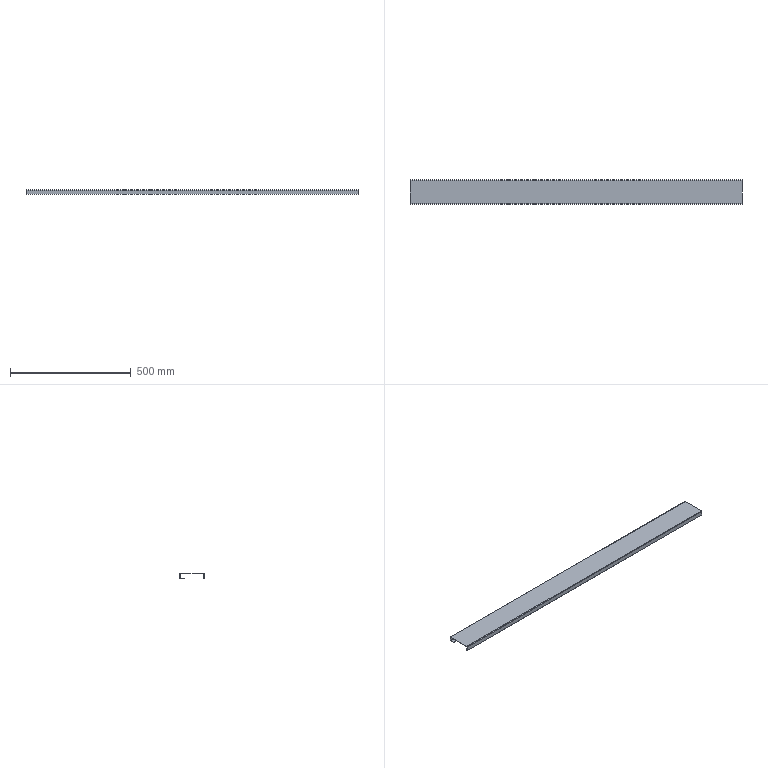Part | STEP file | E3-中转釜护栏6踢脚Plate | 1 solid | 18 faces | box 1375 x 100 x 20 mm | volume 316071 mm3 | plane 12 | cylinder 6 | commonest cylinder face diameters 2 x3 5 x3
STEP:
#1=CARTESIAN_POINT('',(0.,0.,0.));
#2=DIRECTION('',(0.,0.,1.));
#3=DIRECTION('',(1.,0.,0.));
#4=AXIS2_PLACEMENT_3D('',#1,#2,#3);
#5=CARTESIAN_POINT('',(-687.5,1.5,-2.5));
#6=VERTEX_POINT('',#5);
#7=CARTESIAN_POINT('',(-687.5,1.5,-20.));
#8=VERTEX_POINT('',#7);
#9=CARTESIAN_POINT('',(-687.5,1.5,-2.5));
#10=DIRECTION('',(0.,0.,-1.));
#11=VECTOR('',#10,1.);
#12=LINE('',#9,#11);
#13=CARTESIAN_POINT('',(687.5,1.5,-2.5));
#14=DIRECTION('',(0.,-1.,0.));
#15=DIRECTION('',(0.,0.,1.));
#16=AXIS2_PLACEMENT_3D('',#13,#14,#15);
#17=PLANE('',#16);
#18=CARTESIAN_POINT('',(0.,1375.));
#19=DIRECTION('',(-1.,0.));
#20=VECTOR('',#19,1.);
#21=LINE('',#18,#20);
#22=(GEOMETRIC_REPRESENTATION_CONTEXT(2)PARAMETRIC_REPRESENTATION_CONTEXT()REPRESENTATION_CONTEXT('',''));
#23=DEFINITIONAL_REPRESENTATION('',(#21),#22);
#24=PCURVE('',#17,#23);
#25=CARTESIAN_POINT('',(-687.5,2.5,-2.5));
#26=DIRECTION('',(-1.,0.,0.));
#27=DIRECTION('',(0.,0.,-1.));
#28=AXIS2_PLACEMENT_3D('',#25,#26,#27);
#29=PLANE('',#28);
#30=CARTESIAN_POINT('',(0.,1.));
#31=DIRECTION('',(1.,0.));
#32=VECTOR('',#31,1.);
#33=LINE('',#30,#32);
#34=(GEOMETRIC_REPRESENTATION_CONTEXT(2)PARAMETRIC_REPRESENTATION_CONTEXT()REPRESENTATION_CONTEXT('',''));
#35=DEFINITIONAL_REPRESENTATION('',(#33),#34);
#36=PCURVE('',#29,#35);
#37=SURFACE_CURVE('',#12,(#24,#36),.PCURVE_S1.);
#38=EDGE_CURVE('',#6,#8,#37,.T.);
#39=ORIENTED_EDGE('',*,*,#38,.F.);
#40=CARTESIAN_POINT('',(687.5,1.5,-2.5));
#41=VERTEX_POINT('',#40);
#42=CARTESIAN_POINT('',(687.5,1.5,-2.5));
#43=DIRECTION('',(-1.,0.,0.));
#44=VECTOR('',#43,1.);
#45=LINE('',#42,#44);
#46=CARTESIAN_POINT('',(0.,0.));
#47=DIRECTION('',(0.,1.));
#48=VECTOR('',#47,1.);
#49=LINE('',#46,#48);
#50=(GEOMETRIC_REPRESENTATION_CONTEXT(2)PARAMETRIC_REPRESENTATION_CONTEXT()REPRESENTATION_CONTEXT('',''));
#51=DEFINITIONAL_REPRESENTATION('',(#49),#50);
#52=PCURVE('',#17,#51);
#53=CARTESIAN_POINT('',(687.5,2.5,-2.5));
#54=DIRECTION('',(-1.,0.,0.));
#55=DIRECTION('',(0.,0.,-1.));
#56=AXIS2_PLACEMENT_3D('',#53,#54,#55);
#57=CYLINDRICAL_SURFACE('',#56,1.);
#58=CARTESIAN_POINT('',(1.571,0.));
#59=DIRECTION('',(0.,1.));
#60=VECTOR('',#59,1.);
#61=LINE('',#58,#60);
#62=(GEOMETRIC_REPRESENTATION_CONTEXT(2)PARAMETRIC_REPRESENTATION_CONTEXT()REPRESENTATION_CONTEXT('',''));
#63=DEFINITIONAL_REPRESENTATION('',(#61),#62);
#64=PCURVE('',#57,#63);
#65=SURFACE_CURVE('',#45,(#52,#64),.PCURVE_S1.);
#66=EDGE_CURVE('',#41,#6,#65,.T.);
#67=ORIENTED_EDGE('',*,*,#66,.F.);
#68=CARTESIAN_POINT('',(687.5,1.5,-20.));
#69=VERTEX_POINT('',#68);
#70=CARTESIAN_POINT('',(687.5,1.5,-2.5));
#71=DIRECTION('',(0.,0.,-1.));
#72=VECTOR('',#71,1.);
#73=LINE('',#70,#72);
#74=CARTESIAN_POINT('',(0.,0.));
#75=DIRECTION('',(-1.,0.));
#76=VECTOR('',#75,1.);
#77=LINE('',#74,#76);
#78=(GEOMETRIC_REPRESENTATION_CONTEXT(2)PARAMETRIC_REPRESENTATION_CONTEXT()REPRESENTATION_CONTEXT('',''));
#79=DEFINITIONAL_REPRESENTATION('',(#77),#78);
#80=PCURVE('',#17,#79);
#81=CARTESIAN_POINT('',(687.5,2.5,-2.5));
#82=DIRECTION('',(-1.,0.,0.));
#83=DIRECTION('',(0.,0.,-1.));
#84=AXIS2_PLACEMENT_3D('',#81,#82,#83);
#85=PLANE('',#84);
#86=CARTESIAN_POINT('',(0.,1.));
#87=DIRECTION('',(1.,0.));
#88=VECTOR('',#87,1.);
#89=LINE('',#86,#88);
#90=(GEOMETRIC_REPRESENTATION_CONTEXT(2)PARAMETRIC_REPRESENTATION_CONTEXT()REPRESENTATION_CONTEXT('',''));
#91=DEFINITIONAL_REPRESENTATION('',(#89),#90);
#92=PCURVE('',#85,#91);
#93=SURFACE_CURVE('',#73,(#80,#92),.PCURVE_S1.);
#94=EDGE_CURVE('',#41,#69,#93,.T.);
#95=ORIENTED_EDGE('',*,*,#94,.T.);
#96=CARTESIAN_POINT('',(687.5,1.5,-20.));
#97=DIRECTION('',(-1.,0.,0.));
#98=VECTOR('',#97,1.);
#99=LINE('',#96,#98);
#100=CARTESIAN_POINT('',(-17.5,0.));
#101=DIRECTION('',(0.,1.));
#102=VECTOR('',#101,1.);
#103=LINE('',#100,#102);
#104=(GEOMETRIC_REPRESENTATION_CONTEXT(2)PARAMETRIC_REPRESENTATION_CONTEXT()REPRESENTATION_CONTEXT('',''));
#105=DEFINITIONAL_REPRESENTATION('',(#103),#104);
#106=PCURVE('',#17,#105);
#107=CARTESIAN_POINT('',(687.5,0.,-20.));
#108=DIRECTION('',(0.,0.,-1.));
#109=DIRECTION('',(1.,0.,0.));
#110=AXIS2_PLACEMENT_3D('',#107,#108,#109);
#111=PLANE('',#110);
#112=CARTESIAN_POINT('',(0.,-1.5));
#113=DIRECTION('',(-1.,0.));
#114=VECTOR('',#113,1.);
#115=LINE('',#112,#114);
#116=(GEOMETRIC_REPRESENTATION_CONTEXT(2)PARAMETRIC_REPRESENTATION_CONTEXT()REPRESENTATION_CONTEXT('',''));
#117=DEFINITIONAL_REPRESENTATION('',(#115),#116);
#118=PCURVE('',#111,#117);
#119=SURFACE_CURVE('',#99,(#106,#118),.PCURVE_S1.);
#120=EDGE_CURVE('',#69,#8,#119,.T.);
#121=ORIENTED_EDGE('',*,*,#120,.T.);
#122=EDGE_LOOP('',(#39,#67,#95,#121));
#123=FACE_BOUND('',#122,.T.);
#124=ADVANCED_FACE('',(#123),#17,.F.);
#125=CARTESIAN_POINT('',(-687.5,0.,-20.));
#126=VERTEX_POINT('',#125);
#127=CARTESIAN_POINT('',(-687.5,0.,-20.));
#128=DIRECTION('',(0.,1.,0.));
#129=VECTOR('',#128,1.);
#130=LINE('',#127,#129);
#131=CARTESIAN_POINT('',(-1375.,0.));
#132=DIRECTION('',(0.,-1.));
#133=VECTOR('',#132,1.);
#134=LINE('',#131,#133);
#135=(GEOMETRIC_REPRESENTATION_CONTEXT(2)PARAMETRIC_REPRESENTATION_CONTEXT()REPRESENTATION_CONTEXT('',''));
#136=DEFINITIONAL_REPRESENTATION('',(#134),#135);
#137=PCURVE('',#111,#136);
#138=CARTESIAN_POINT('',(17.5,2.5));
#139=DIRECTION('',(0.,-1.));
#140=VECTOR('',#139,1.);
#141=LINE('',#138,#140);
#142=(GEOMETRIC_REPRESENTATION_CONTEXT(2)PARAMETRIC_REPRESENTATION_CONTEXT()REPRESENTATION_CONTEXT('',''));
#143=DEFINITIONAL_REPRESENTATION('',(#141),#142);
#144=PCURVE('',#29,#143);
#145=SURFACE_CURVE('',#130,(#137,#144),.PCURVE_S1.);
#146=EDGE_CURVE('',#126,#8,#145,.T.);
#147=ORIENTED_EDGE('',*,*,#146,.T.);
#148=ORIENTED_EDGE('',*,*,#120,.F.);
#149=CARTESIAN_POINT('',(687.5,0.,-20.));
#150=VERTEX_POINT('',#149);
#151=CARTESIAN_POINT('',(687.5,0.,-20.));
#152=DIRECTION('',(0.,1.,0.));
#153=VECTOR('',#152,1.);
#154=LINE('',#151,#153);
#155=CARTESIAN_POINT('',(0.,0.));
#156=DIRECTION('',(0.,-1.));
#157=VECTOR('',#156,1.);
#158=LINE('',#155,#157);
#159=(GEOMETRIC_REPRESENTATION_CONTEXT(2)PARAMETRIC_REPRESENTATION_CONTEXT()REPRESENTATION_CONTEXT('',''));
#160=DEFINITIONAL_REPRESENTATION('',(#158),#159);
#161=PCURVE('',#111,#160);
#162=CARTESIAN_POINT('',(17.5,2.5));
#163=DIRECTION('',(0.,-1.));
#164=VECTOR('',#163,1.);
#165=LINE('',#162,#164);
#166=(GEOMETRIC_REPRESENTATION_CONTEXT(2)PARAMETRIC_REPRESENTATION_CONTEXT()REPRESENTATION_CONTEXT('',''));
#167=DEFINITIONAL_REPRESENTATION('',(#165),#166);
#168=PCURVE('',#85,#167);
#169=SURFACE_CURVE('',#154,(#161,#168),.PCURVE_S1.);
#170=EDGE_CURVE('',#150,#69,#169,.T.);
#171=ORIENTED_EDGE('',*,*,#170,.F.);
#172=CARTESIAN_POINT('',(687.5,0.,-20.));
#173=DIRECTION('',(-1.,0.,0.));
#174=VECTOR('',#173,1.);
#175=LINE('',#172,#174);
#176=CARTESIAN_POINT('',(0.,0.));
#177=DIRECTION('',(-1.,0.));
#178=VECTOR('',#177,1.);
#179=LINE('',#176,#178);
#180=(GEOMETRIC_REPRESENTATION_CONTEXT(2)PARAMETRIC_REPRESENTATION_CONTEXT()REPRESENTATION_CONTEXT('',''));
#181=DEFINITIONAL_REPRESENTATION('',(#179),#180);
#182=PCURVE('',#111,#181);
#183=CARTESIAN_POINT('',(687.5,0.,-2.5));
#184=DIRECTION('',(0.,-1.,0.));
#185=DIRECTION('',(0.,0.,1.));
#186=AXIS2_PLACEMENT_3D('',#183,#184,#185);
#187=PLANE('',#186);
#188=CARTESIAN_POINT('',(-17.5,0.));
#189=DIRECTION('',(0.,1.));
#190=VECTOR('',#189,1.);
#191=LINE('',#188,#190);
#192=(GEOMETRIC_REPRESENTATION_CONTEXT(2)PARAMETRIC_REPRESENTATION_CONTEXT()REPRESENTATION_CONTEXT('',''));
#193=DEFINITIONAL_REPRESENTATION('',(#191),#192);
#194=PCURVE('',#187,#193);
#195=SURFACE_CURVE('',#175,(#182,#194),.PCURVE_S1.);
#196=EDGE_CURVE('',#150,#126,#195,.T.);
#197=ORIENTED_EDGE('',*,*,#196,.T.);
#198=EDGE_LOOP('',(#147,#148,#171,#197));
#199=FACE_BOUND('',#198,.T.);
#200=ADVANCED_FACE('',(#199),#111,.T.);
#201=CARTESIAN_POINT('',(-687.5,0.,-2.5));
#202=VERTEX_POINT('',#201);
#203=CARTESIAN_POINT('',(-687.5,0.,-2.5));
#204=DIRECTION('',(0.,0.,-1.));
#205=VECTOR('',#204,1.);
#206=LINE('',#203,#205);
#207=CARTESIAN_POINT('',(0.,1375.));
#208=DIRECTION('',(-1.,0.));
#209=VECTOR('',#208,1.);
#210=LINE('',#207,#209);
#211=(GEOMETRIC_REPRESENTATION_CONTEXT(2)PARAMETRIC_REPRESENTATION_CONTEXT()REPRESENTATION_CONTEXT('',''));
#212=DEFINITIONAL_REPRESENTATION('',(#210),#211);
#213=PCURVE('',#187,#212);
#214=CARTESIAN_POINT('',(0.,2.5));
#215=DIRECTION('',(1.,0.));
#216=VECTOR('',#215,1.);
#217=LINE('',#214,#216);
#218=(GEOMETRIC_REPRESENTATION_CONTEXT(2)PARAMETRIC_REPRESENTATION_CONTEXT()REPRESENTATION_CONTEXT('',''));
#219=DEFINITIONAL_REPRESENTATION('',(#217),#218);
#220=PCURVE('',#29,#219);
#221=SURFACE_CURVE('',#206,(#213,#220),.PCURVE_S1.);
#222=EDGE_CURVE('',#202,#126,#221,.T.);
#223=ORIENTED_EDGE('',*,*,#222,.T.);
#224=ORIENTED_EDGE('',*,*,#196,.F.);
#225=CARTESIAN_POINT('',(687.5,0.,-2.5));
#226=VERTEX_POINT('',#225);
#227=CARTESIAN_POINT('',(687.5,0.,-2.5));
#228=DIRECTION('',(0.,0.,-1.));
#229=VECTOR('',#228,1.);
#230=LINE('',#227,#229);
#231=CARTESIAN_POINT('',(0.,0.));
#232=DIRECTION('',(-1.,0.));
#233=VECTOR('',#232,1.);
#234=LINE('',#231,#233);
#235=(GEOMETRIC_REPRESENTATION_CONTEXT(2)PARAMETRIC_REPRESENTATION_CONTEXT()REPRESENTATION_CONTEXT('',''));
#236=DEFINITIONAL_REPRESENTATION('',(#234),#235);
#237=PCURVE('',#187,#236);
#238=CARTESIAN_POINT('',(0.,2.5));
#239=DIRECTION('',(1.,0.));
#240=VECTOR('',#239,1.);
#241=LINE('',#238,#240);
#242=(GEOMETRIC_REPRESENTATION_CONTEXT(2)PARAMETRIC_REPRESENTATION_CONTEXT()REPRESENTATION_CONTEXT('',''));
#243=DEFINITIONAL_REPRESENTATION('',(#241),#242);
#244=PCURVE('',#85,#243);
#245=SURFACE_CURVE('',#230,(#237,#244),.PCURVE_S1.);
#246=EDGE_CURVE('',#226,#150,#245,.T.);
#247=ORIENTED_EDGE('',*,*,#246,.F.);
#248=CARTESIAN_POINT('',(687.5,0.,-2.5));
#249=DIRECTION('',(-1.,0.,0.));
#250=VECTOR('',#249,1.);
#251=LINE('',#248,#250);
#252=CARTESIAN_POINT('',(0.,0.));
#253=DIRECTION('',(0.,1.));
#254=VECTOR('',#253,1.);
#255=LINE('',#252,#254);
#256=(GEOMETRIC_REPRESENTATION_CONTEXT(2)PARAMETRIC_REPRESENTATION_CONTEXT()REPRESENTATION_CONTEXT('',''));
#257=DEFINITIONAL_REPRESENTATION('',(#255),#256);
#258=PCURVE('',#187,#257);
#259=CARTESIAN_POINT('',(687.5,2.5,-2.5));
#260=DIRECTION('',(-1.,0.,0.));
#261=DIRECTION('',(0.,0.,-1.));
#262=AXIS2_PLACEMENT_3D('',#259,#260,#261);
#263=CYLINDRICAL_SURFACE('',#262,2.5);
#264=CARTESIAN_POINT('',(1.571,0.));
#265=DIRECTION('',(0.,1.));
#266=VECTOR('',#265,1.);
#267=LINE('',#264,#266);
#268=(GEOMETRIC_REPRESENTATION_CONTEXT(2)PARAMETRIC_REPRESENTATION_CONTEXT()REPRESENTATION_CONTEXT('',''));
#269=DEFINITIONAL_REPRESENTATION('',(#267),#268);
#270=PCURVE('',#263,#269);
#271=SURFACE_CURVE('',#251,(#258,#270),.PCURVE_S1.);
#272=EDGE_CURVE('',#226,#202,#271,.T.);
#273=ORIENTED_EDGE('',*,*,#272,.T.);
#274=EDGE_LOOP('',(#223,#224,#247,#273));
#275=FACE_BOUND('',#274,.T.);
#276=ADVANCED_FACE('',(#275),#187,.T.);
#277=CARTESIAN_POINT('',(-687.5,2.5,0.));
#278=VERTEX_POINT('',#277);
#279=CARTESIAN_POINT('',(-687.5,2.5,-2.5));
#280=DIRECTION('',(1.,0.,0.));
#281=DIRECTION('',(0.,0.,-1.));
#282=AXIS2_PLACEMENT_3D('',#279,#280,#281);
#283=CIRCLE('',#282,2.5);
#284=CARTESIAN_POINT('',(6.283,1375.));
#285=DIRECTION('',(-1.,0.));
#286=VECTOR('',#285,1.);
#287=LINE('',#284,#286);
#288=(GEOMETRIC_REPRESENTATION_CONTEXT(2)PARAMETRIC_REPRESENTATION_CONTEXT()REPRESENTATION_CONTEXT('',''));
#289=DEFINITIONAL_REPRESENTATION('',(#287),#288);
#290=PCURVE('',#263,#289);
#291=CARTESIAN_POINT('',(2.5,0.));
#292=CARTESIAN_POINT('',(2.5,-4.33));
#293=CARTESIAN_POINT('',(-1.25,-2.165));
#294=CARTESIAN_POINT('',(-5.,0.));
#295=CARTESIAN_POINT('',(-1.25,2.165));
#296=CARTESIAN_POINT('',(2.5,4.33));
#297=CARTESIAN_POINT('',(2.5,0.));
#298=(BOUNDED_CURVE()B_SPLINE_CURVE(2,(#291,#292,#293,#294,#295,#296,#297),.UNSPECIFIED.,.T.,.F.)B_SPLINE_CURVE_WITH_KNOTS((1,2,2,2,2,1),(-2.094,0.,2.094,4.189,6.283,8.378),.UNSPECIFIED.)CURVE()GEOMETRIC_REPRESENTATION_ITEM()RATIONAL_B_SPLINE_CURVE((1.,0.5,1.,0.5,1.,0.5,1.))REPRESENTATION_ITEM(''));
#299=(GEOMETRIC_REPRESENTATION_CONTEXT(2)PARAMETRIC_REPRESENTATION_CONTEXT()REPRESENTATION_CONTEXT('',''));
#300=DEFINITIONAL_REPRESENTATION('',(#298),#299);
#301=PCURVE('',#29,#300);
#302=SURFACE_CURVE('',#283,(#290,#301),.PCURVE_S1.);
#303=EDGE_CURVE('',#278,#202,#302,.T.);
#304=ORIENTED_EDGE('',*,*,#303,.T.);
#305=ORIENTED_EDGE('',*,*,#272,.F.);
#306=CARTESIAN_POINT('',(687.5,2.5,0.));
#307=VERTEX_POINT('',#306);
#308=CARTESIAN_POINT('',(687.5,2.5,-2.5));
#309=DIRECTION('',(1.,0.,0.));
#310=DIRECTION('',(0.,0.,-1.));
#311=AXIS2_PLACEMENT_3D('',#308,#309,#310);
#312=CIRCLE('',#311,2.5);
#313=CARTESIAN_POINT('',(6.283,0.));
#314=DIRECTION('',(-1.,0.));
#315=VECTOR('',#314,1.);
#316=LINE('',#313,#315);
#317=(GEOMETRIC_REPRESENTATION_CONTEXT(2)PARAMETRIC_REPRESENTATION_CONTEXT()REPRESENTATION_CONTEXT('',''));
#318=DEFINITIONAL_REPRESENTATION('',(#316),#317);
#319=PCURVE('',#263,#318);
#320=CARTESIAN_POINT('',(2.5,0.));
#321=CARTESIAN_POINT('',(2.5,-4.33));
#322=CARTESIAN_POINT('',(-1.25,-2.165));
#323=CARTESIAN_POINT('',(-5.,0.));
#324=CARTESIAN_POINT('',(-1.25,2.165));
#325=CARTESIAN_POINT('',(2.5,4.33));
#326=CARTESIAN_POINT('',(2.5,0.));
#327=(BOUNDED_CURVE()B_SPLINE_CURVE(2,(#320,#321,#322,#323,#324,#325,#326),.UNSPECIFIED.,.T.,.F.)B_SPLINE_CURVE_WITH_KNOTS((1,2,2,2,2,1),(-2.094,0.,2.094,4.189,6.283,8.378),.UNSPECIFIED.)CURVE()GEOMETRIC_REPRESENTATION_ITEM()RATIONAL_B_SPLINE_CURVE((1.,0.5,1.,0.5,1.,0.5,1.))REPRESENTATION_ITEM(''));
#328=(GEOMETRIC_REPRESENTATION_CONTEXT(2)PARAMETRIC_REPRESENTATION_CONTEXT()REPRESENTATION_CONTEXT('',''));
#329=DEFINITIONAL_REPRESENTATION('',(#327),#328);
#330=PCURVE('',#85,#329);
#331=SURFACE_CURVE('',#312,(#319,#330),.PCURVE_S1.);
#332=EDGE_CURVE('',#307,#226,#331,.T.);
#333=ORIENTED_EDGE('',*,*,#332,.F.);
#334=CARTESIAN_POINT('',(687.5,2.5,0.));
#335=DIRECTION('',(-1.,0.,0.));
#336=VECTOR('',#335,1.);
#337=LINE('',#334,#336);
#338=CARTESIAN_POINT('',(3.142,0.));
#339=DIRECTION('',(0.,1.));
#340=VECTOR('',#339,1.);
#341=LINE('',#338,#340);
#342=(GEOMETRIC_REPRESENTATION_CONTEXT(2)PARAMETRIC_REPRESENTATION_CONTEXT()REPRESENTATION_CONTEXT('',''));
#343=DEFINITIONAL_REPRESENTATION('',(#341),#342);
#344=PCURVE('',#263,#343);
#345=CARTESIAN_POINT('',(687.5,2.5,0.));
#346=DIRECTION('',(0.,0.,1.));
#347=DIRECTION('',(-1.,0.,0.));
#348=AXIS2_PLACEMENT_3D('',#345,#346,#347);
#349=PLANE('',#348);
#350=CARTESIAN_POINT('',(0.,0.));
#351=DIRECTION('',(1.,0.));
#352=VECTOR('',#351,1.);
#353=LINE('',#350,#352);
#354=(GEOMETRIC_REPRESENTATION_CONTEXT(2)PARAMETRIC_REPRESENTATION_CONTEXT()REPRESENTATION_CONTEXT('',''));
#355=DEFINITIONAL_REPRESENTATION('',(#353),#354);
#356=PCURVE('',#349,#355);
#357=SURFACE_CURVE('',#337,(#344,#356),.PCURVE_S1.);
#358=EDGE_CURVE('',#307,#278,#357,.T.);
#359=ORIENTED_EDGE('',*,*,#358,.T.);
#360=EDGE_LOOP('',(#304,#305,#333,#359));
#361=FACE_BOUND('',#360,.T.);
#362=ADVANCED_FACE('',(#361),#263,.T.);
#363=CARTESIAN_POINT('',(-687.5,97.5,0.));
#364=VERTEX_POINT('',#363);
#365=CARTESIAN_POINT('',(-687.5,2.5,0.));
#366=DIRECTION('',(0.,-1.,0.));
#367=VECTOR('',#366,1.);
#368=LINE('',#365,#367);
#369=CARTESIAN_POINT('',(1375.,0.));
#370=DIRECTION('',(0.,1.));
#371=VECTOR('',#370,1.);
#372=LINE('',#369,#371);
#373=(GEOMETRIC_REPRESENTATION_CONTEXT(2)PARAMETRIC_REPRESENTATION_CONTEXT()REPRESENTATION_CONTEXT('',''));
#374=DEFINITIONAL_REPRESENTATION('',(#372),#373);
#375=PCURVE('',#349,#374);
#376=CARTESIAN_POINT('',(-2.5,0.));
#377=DIRECTION('',(0.,1.));
#378=VECTOR('',#377,1.);
#379=LINE('',#376,#378);
#380=(GEOMETRIC_REPRESENTATION_CONTEXT(2)PARAMETRIC_REPRESENTATION_CONTEXT()REPRESENTATION_CONTEXT('',''));
#381=DEFINITIONAL_REPRESENTATION('',(#379),#380);
#382=PCURVE('',#29,#381);
#383=SURFACE_CURVE('',#368,(#375,#382),.PCURVE_S1.);
#384=EDGE_CURVE('',#364,#278,#383,.T.);
#385=ORIENTED_EDGE('',*,*,#384,.T.);
#386=ORIENTED_EDGE('',*,*,#358,.F.);
#387=CARTESIAN_POINT('',(687.5,97.5,0.));
#388=VERTEX_POINT('',#387);
#389=CARTESIAN_POINT('',(687.5,2.5,0.));
#390=DIRECTION('',(0.,-1.,0.));
#391=VECTOR('',#390,1.);
#392=LINE('',#389,#391);
#393=CARTESIAN_POINT('',(0.,0.));
#394=DIRECTION('',(0.,1.));
#395=VECTOR('',#394,1.);
#396=LINE('',#393,#395);
#397=(GEOMETRIC_REPRESENTATION_CONTEXT(2)PARAMETRIC_REPRESENTATION_CONTEXT()REPRESENTATION_CONTEXT('',''));
#398=DEFINITIONAL_REPRESENTATION('',(#396),#397);
#399=PCURVE('',#349,#398);
#400=CARTESIAN_POINT('',(-2.5,0.));
#401=DIRECTION('',(0.,1.));
#402=VECTOR('',#401,1.);
#403=LINE('',#400,#402);
#404=(GEOMETRIC_REPRESENTATION_CONTEXT(2)PARAMETRIC_REPRESENTATION_CONTEXT()REPRESENTATION_CONTEXT('',''));
#405=DEFINITIONAL_REPRESENTATION('',(#403),#404);
#406=PCURVE('',#85,#405);
#407=SURFACE_CURVE('',#392,(#399,#406),.PCURVE_S1.);
#408=EDGE_CURVE('',#388,#307,#407,.T.);
#409=ORIENTED_EDGE('',*,*,#408,.F.);
#410=CARTESIAN_POINT('',(687.5,97.5,0.));
#411=DIRECTION('',(-1.,0.,0.));
#412=VECTOR('',#411,1.);
#413=LINE('',#410,#412);
#414=CARTESIAN_POINT('',(0.,-95.));
#415=DIRECTION('',(1.,0.));
#416=VECTOR('',#415,1.);
#417=LINE('',#414,#416);
#418=(GEOMETRIC_REPRESENTATION_CONTEXT(2)PARAMETRIC_REPRESENTATION_CONTEXT()REPRESENTATION_CONTEXT('',''));
#419=DEFINITIONAL_REPRESENTATION('',(#417),#418);
#420=PCURVE('',#349,#419);
#421=CARTESIAN_POINT('',(687.5,97.5,-2.5));
#422=DIRECTION('',(-1.,0.,0.));
#423=DIRECTION('',(0.,0.,-1.));
#424=AXIS2_PLACEMENT_3D('',#421,#422,#423);
#425=CYLINDRICAL_SURFACE('',#424,2.5);
#426=CARTESIAN_POINT('',(3.142,0.));
#427=DIRECTION('',(0.,1.));
#428=VECTOR('',#427,1.);
#429=LINE('',#426,#428);
#430=(GEOMETRIC_REPRESENTATION_CONTEXT(2)PARAMETRIC_REPRESENTATION_CONTEXT()REPRESENTATION_CONTEXT('',''));
#431=DEFINITIONAL_REPRESENTATION('',(#429),#430);
#432=PCURVE('',#425,#431);
#433=SURFACE_CURVE('',#413,(#420,#432),.PCURVE_S1.);
#434=EDGE_CURVE('',#388,#364,#433,.T.);
#435=ORIENTED_EDGE('',*,*,#434,.T.);
#436=EDGE_LOOP('',(#385,#386,#409,#435));
#437=FACE_BOUND('',#436,.T.);
#438=ADVANCED_FACE('',(#437),#349,.T.);
#439=CARTESIAN_POINT('',(-687.5,100.,-2.5));
#440=VERTEX_POINT('',#439);
#441=CARTESIAN_POINT('',(-687.5,97.5,-2.5));
#442=DIRECTION('',(1.,0.,0.));
#443=DIRECTION('',(0.,0.,1.));
#444=AXIS2_PLACEMENT_3D('',#441,#442,#443);
#445=CIRCLE('',#444,2.5);
#446=CARTESIAN_POINT('',(9.425,1375.));
#447=DIRECTION('',(-1.,0.));
#448=VECTOR('',#447,1.);
#449=LINE('',#446,#448);
#450=(GEOMETRIC_REPRESENTATION_CONTEXT(2)PARAMETRIC_REPRESENTATION_CONTEXT()REPRESENTATION_CONTEXT('',''));
#451=DEFINITIONAL_REPRESENTATION('',(#449),#450);
#452=PCURVE('',#425,#451);
#453=CARTESIAN_POINT('',(-2.5,-95.));
#454=CARTESIAN_POINT('',(-2.5,-90.67));
#455=CARTESIAN_POINT('',(1.25,-92.835));
#456=CARTESIAN_POINT('',(5.,-95.));
#457=CARTESIAN_POINT('',(1.25,-97.165));
#458=CARTESIAN_POINT('',(-2.5,-99.33));
#459=CARTESIAN_POINT('',(-2.5,-95.));
#460=(BOUNDED_CURVE()B_SPLINE_CURVE(2,(#453,#454,#455,#456,#457,#458,#459),.UNSPECIFIED.,.T.,.F.)B_SPLINE_CURVE_WITH_KNOTS((1,2,2,2,2,1),(-2.094,0.,2.094,4.189,6.283,8.378),.UNSPECIFIED.)CURVE()GEOMETRIC_REPRESENTATION_ITEM()RATIONAL_B_SPLINE_CURVE((1.,0.5,1.,0.5,1.,0.5,1.))REPRESENTATION_ITEM(''));
#461=(GEOMETRIC_REPRESENTATION_CONTEXT(2)PARAMETRIC_REPRESENTATION_CONTEXT()REPRESENTATION_CONTEXT('',''));
#462=DEFINITIONAL_REPRESENTATION('',(#460),#461);
#463=PCURVE('',#29,#462);
#464=SURFACE_CURVE('',#445,(#452,#463),.PCURVE_S1.);
#465=EDGE_CURVE('',#440,#364,#464,.T.);
#466=ORIENTED_EDGE('',*,*,#465,.T.);
#467=ORIENTED_EDGE('',*,*,#434,.F.);
#468=CARTESIAN_POINT('',(687.5,100.,-2.5));
#469=VERTEX_POINT('',#468);
#470=CARTESIAN_POINT('',(687.5,97.5,-2.5));
#471=DIRECTION('',(1.,0.,0.));
#472=DIRECTION('',(0.,0.,1.));
#473=AXIS2_PLACEMENT_3D('',#470,#471,#472);
#474=CIRCLE('',#473,2.5);
#475=CARTESIAN_POINT('',(9.425,0.));
#476=DIRECTION('',(-1.,0.));
#477=VECTOR('',#476,1.);
#478=LINE('',#475,#477);
#479=(GEOMETRIC_REPRESENTATION_CONTEXT(2)PARAMETRIC_REPRESENTATION_CONTEXT()REPRESENTATION_CONTEXT('',''));
#480=DEFINITIONAL_REPRESENTATION('',(#478),#479);
#481=PCURVE('',#425,#480);
#482=CARTESIAN_POINT('',(-2.5,-95.));
#483=CARTESIAN_POINT('',(-2.5,-90.67));
#484=CARTESIAN_POINT('',(1.25,-92.835));
#485=CARTESIAN_POINT('',(5.,-95.));
#486=CARTESIAN_POINT('',(1.25,-97.165));
#487=CARTESIAN_POINT('',(-2.5,-99.33));
#488=CARTESIAN_POINT('',(-2.5,-95.));
#489=(BOUNDED_CURVE()B_SPLINE_CURVE(2,(#482,#483,#484,#485,#486,#487,#488),.UNSPECIFIED.,.T.,.F.)B_SPLINE_CURVE_WITH_KNOTS((1,2,2,2,2,1),(-2.094,0.,2.094,4.189,6.283,8.378),.UNSPECIFIED.)CURVE()GEOMETRIC_REPRESENTATION_ITEM()RATIONAL_B_SPLINE_CURVE((1.,0.5,1.,0.5,1.,0.5,1.))REPRESENTATION_ITEM(''));
#490=(GEOMETRIC_REPRESENTATION_CONTEXT(2)PARAMETRIC_REPRESENTATION_CONTEXT()REPRESENTATION_CONTEXT('',''));
#491=DEFINITIONAL_REPRESENTATION('',(#489),#490);
#492=PCURVE('',#85,#491);
#493=SURFACE_CURVE('',#474,(#481,#492),.PCURVE_S1.);
#494=EDGE_CURVE('',#469,#388,#493,.T.);
#495=ORIENTED_EDGE('',*,*,#494,.F.);
#496=CARTESIAN_POINT('',(687.5,100.,-2.5));
#497=DIRECTION('',(-1.,0.,0.));
#498=VECTOR('',#497,1.);
#499=LINE('',#496,#498);
#500=CARTESIAN_POINT('',(4.712,0.));
#501=DIRECTION('',(0.,1.));
#502=VECTOR('',#501,1.);
#503=LINE('',#500,#502);
#504=(GEOMETRIC_REPRESENTATION_CONTEXT(2)PARAMETRIC_REPRESENTATION_CONTEXT()REPRESENTATION_CONTEXT('',''));
#505=DEFINITIONAL_REPRESENTATION('',(#503),#504);
#506=PCURVE('',#425,#505);
#507=CARTESIAN_POINT('',(687.5,100.,-2.5));
#508=DIRECTION('',(0.,1.,0.));
#509=DIRECTION('',(0.,0.,-1.));
#510=AXIS2_PLACEMENT_3D('',#507,#508,#509);
#511=PLANE('',#510);
#512=CARTESIAN_POINT('',(0.,0.));
#513=DIRECTION('',(0.,1.));
#514=VECTOR('',#513,1.);
#515=LINE('',#512,#514);
#516=(GEOMETRIC_REPRESENTATION_CONTEXT(2)PARAMETRIC_REPRESENTATION_CONTEXT()REPRESENTATION_CONTEXT('',''));
#517=DEFINITIONAL_REPRESENTATION('',(#515),#516);
#518=PCURVE('',#511,#517);
#519=SURFACE_CURVE('',#499,(#506,#518),.PCURVE_S1.);
#520=EDGE_CURVE('',#469,#440,#519,.T.);
#521=ORIENTED_EDGE('',*,*,#520,.T.);
#522=EDGE_LOOP('',(#466,#467,#495,#521));
#523=FACE_BOUND('',#522,.T.);
#524=ADVANCED_FACE('',(#523),#425,.T.);
#525=CARTESIAN_POINT('',(-687.5,100.,-17.5));
#526=VERTEX_POINT('',#525);
#527=CARTESIAN_POINT('',(-687.5,100.,-2.5));
#528=DIRECTION('',(0.,0.,1.));
#529=VECTOR('',#528,1.);
#530=LINE('',#527,#529);
#531=CARTESIAN_POINT('',(0.,1375.));
#532=DIRECTION('',(-1.,0.));
#533=VECTOR('',#532,1.);
#534=LINE('',#531,#533);
#535=(GEOMETRIC_REPRESENTATION_CONTEXT(2)PARAMETRIC_REPRESENTATION_CONTEXT()REPRESENTATION_CONTEXT('',''));
#536=DEFINITIONAL_REPRESENTATION('',(#534),#535);
#537=PCURVE('',#511,#536);
#538=CARTESIAN_POINT('',(0.,-97.5));
#539=DIRECTION('',(-1.,0.));
#540=VECTOR('',#539,1.);
#541=LINE('',#538,#540);
#542=(GEOMETRIC_REPRESENTATION_CONTEXT(2)PARAMETRIC_REPRESENTATION_CONTEXT()REPRESENTATION_CONTEXT('',''));
#543=DEFINITIONAL_REPRESENTATION('',(#541),#542);
#544=PCURVE('',#29,#543);
#545=SURFACE_CURVE('',#530,(#537,#544),.PCURVE_S1.);
#546=EDGE_CURVE('',#526,#440,#545,.T.);
#547=ORIENTED_EDGE('',*,*,#546,.T.);
#548=ORIENTED_EDGE('',*,*,#520,.F.);
#549=CARTESIAN_POINT('',(687.5,100.,-17.5));
#550=VERTEX_POINT('',#549);
#551=CARTESIAN_POINT('',(687.5,100.,-2.5));
#552=DIRECTION('',(0.,0.,1.));
#553=VECTOR('',#552,1.);
#554=LINE('',#551,#553);
#555=CARTESIAN_POINT('',(0.,0.));
#556=DIRECTION('',(-1.,0.));
#557=VECTOR('',#556,1.);
#558=LINE('',#555,#557);
#559=(GEOMETRIC_REPRESENTATION_CONTEXT(2)PARAMETRIC_REPRESENTATION_CONTEXT()REPRESENTATION_CONTEXT('',''));
#560=DEFINITIONAL_REPRESENTATION('',(#558),#559);
#561=PCURVE('',#511,#560);
#562=CARTESIAN_POINT('',(0.,-97.5));
#563=DIRECTION('',(-1.,0.));
#564=VECTOR('',#563,1.);
#565=LINE('',#562,#564);
#566=(GEOMETRIC_REPRESENTATION_CONTEXT(2)PARAMETRIC_REPRESENTATION_CONTEXT()REPRESENTATION_CONTEXT('',''));
#567=DEFINITIONAL_REPRESENTATION('',(#565),#566);
#568=PCURVE('',#85,#567);
#569=SURFACE_CURVE('',#554,(#561,#568),.PCURVE_S1.);
#570=EDGE_CURVE('',#550,#469,#569,.T.);
#571=ORIENTED_EDGE('',*,*,#570,.F.);
#572=CARTESIAN_POINT('',(687.5,100.,-17.5));
#573=DIRECTION('',(-1.,0.,0.));
#574=VECTOR('',#573,1.);
#575=LINE('',#572,#574);
#576=CARTESIAN_POINT('',(15.,0.));
#577=DIRECTION('',(0.,1.));
#578=VECTOR('',#577,1.);
#579=LINE('',#576,#578);
#580=(GEOMETRIC_REPRESENTATION_CONTEXT(2)PARAMETRIC_REPRESENTATION_CONTEXT()REPRESENTATION_CONTEXT('',''));
#581=DEFINITIONAL_REPRESENTATION('',(#579),#580);
#582=PCURVE('',#511,#581);
#583=CARTESIAN_POINT('',(687.5,97.5,-17.5));
#584=DIRECTION('',(-1.,0.,0.));
#585=DIRECTION('',(0.,0.,-1.));
#586=AXIS2_PLACEMENT_3D('',#583,#584,#585);
#587=CYLINDRICAL_SURFACE('',#586,2.5);
#588=CARTESIAN_POINT('',(4.712,0.));
#589=DIRECTION('',(0.,1.));
#590=VECTOR('',#589,1.);
#591=LINE('',#588,#590);
#592=(GEOMETRIC_REPRESENTATION_CONTEXT(2)PARAMETRIC_REPRESENTATION_CONTEXT()REPRESENTATION_CONTEXT('',''));
#593=DEFINITIONAL_REPRESENTATION('',(#591),#592);
#594=PCURVE('',#587,#593);
#595=SURFACE_CURVE('',#575,(#582,#594),.PCURVE_S1.);
#596=EDGE_CURVE('',#550,#526,#595,.T.);
#597=ORIENTED_EDGE('',*,*,#596,.T.);
#598=EDGE_LOOP('',(#547,#548,#571,#597));
#599=FACE_BOUND('',#598,.T.);
#600=ADVANCED_FACE('',(#599),#511,.T.);
#601=CARTESIAN_POINT('',(-687.5,97.5,-20.));
#602=VERTEX_POINT('',#601);
#603=CARTESIAN_POINT('',(-687.5,97.5,-17.5));
#604=DIRECTION('',(1.,0.,0.));
#605=DIRECTION('',(0.,0.,1.));
#606=AXIS2_PLACEMENT_3D('',#603,#604,#605);
#607=CIRCLE('',#606,2.5);
#608=CARTESIAN_POINT('',(9.425,1375.));
#609=DIRECTION('',(-1.,0.));
#610=VECTOR('',#609,1.);
#611=LINE('',#608,#610);
#612=(GEOMETRIC_REPRESENTATION_CONTEXT(2)PARAMETRIC_REPRESENTATION_CONTEXT()REPRESENTATION_CONTEXT('',''));
#613=DEFINITIONAL_REPRESENTATION('',(#611),#612);
#614=PCURVE('',#587,#613);
#615=CARTESIAN_POINT('',(12.5,-95.));
#616=CARTESIAN_POINT('',(12.5,-90.67));
#617=CARTESIAN_POINT('',(16.25,-92.835));
#618=CARTESIAN_POINT('',(20.,-95.));
#619=CARTESIAN_POINT('',(16.25,-97.165));
#620=CARTESIAN_POINT('',(12.5,-99.33));
#621=CARTESIAN_POINT('',(12.5,-95.));
#622=(BOUNDED_CURVE()B_SPLINE_CURVE(2,(#615,#616,#617,#618,#619,#620,#621),.UNSPECIFIED.,.T.,.F.)B_SPLINE_CURVE_WITH_KNOTS((1,2,2,2,2,1),(-2.094,0.,2.094,4.189,6.283,8.378),.UNSPECIFIED.)CURVE()GEOMETRIC_REPRESENTATION_ITEM()RATIONAL_B_SPLINE_CURVE((1.,0.5,1.,0.5,1.,0.5,1.))REPRESENTATION_ITEM(''));
#623=(GEOMETRIC_REPRESENTATION_CONTEXT(2)PARAMETRIC_REPRESENTATION_CONTEXT()REPRESENTATION_CONTEXT('',''));
#624=DEFINITIONAL_REPRESENTATION('',(#622),#623);
#625=PCURVE('',#29,#624);
#626=SURFACE_CURVE('',#607,(#614,#625),.PCURVE_S1.);
#627=EDGE_CURVE('',#602,#526,#626,.T.);
#628=ORIENTED_EDGE('',*,*,#627,.T.);
#629=ORIENTED_EDGE('',*,*,#596,.F.);
#630=CARTESIAN_POINT('',(687.5,97.5,-20.));
#631=VERTEX_POINT('',#630);
#632=CARTESIAN_POINT('',(687.5,97.5,-17.5));
#633=DIRECTION('',(1.,0.,0.));
#634=DIRECTION('',(0.,0.,1.));
#635=AXIS2_PLACEMENT_3D('',#632,#633,#634);
#636=CIRCLE('',#635,2.5);
#637=CARTESIAN_POINT('',(9.425,0.));
#638=DIRECTION('',(-1.,0.));
#639=VECTOR('',#638,1.);
#640=LINE('',#637,#639);
#641=(GEOMETRIC_REPRESENTATION_CONTEXT(2)PARAMETRIC_REPRESENTATION_CONTEXT()REPRESENTATION_CONTEXT('',''));
#642=DEFINITIONAL_REPRESENTATION('',(#640),#641);
#643=PCURVE('',#587,#642);
#644=CARTESIAN_POINT('',(12.5,-95.));
#645=CARTESIAN_POINT('',(12.5,-90.67));
#646=CARTESIAN_POINT('',(16.25,-92.835));
#647=CARTESIAN_POINT('',(20.,-95.));
#648=CARTESIAN_POINT('',(16.25,-97.165));
#649=CARTESIAN_POINT('',(12.5,-99.33));
#650=CARTESIAN_POINT('',(12.5,-95.));
#651=(BOUNDED_CURVE()B_SPLINE_CURVE(2,(#644,#645,#646,#647,#648,#649,#650),.UNSPECIFIED.,.T.,.F.)B_SPLINE_CURVE_WITH_KNOTS((1,2,2,2,2,1),(-2.094,0.,2.094,4.189,6.283,8.378),.UNSPECIFIED.)CURVE()GEOMETRIC_REPRESENTATION_ITEM()RATIONAL_B_SPLINE_CURVE((1.,0.5,1.,0.5,1.,0.5,1.))REPRESENTATION_ITEM(''));
#652=(GEOMETRIC_REPRESENTATION_CONTEXT(2)PARAMETRIC_REPRESENTATION_CONTEXT()REPRESENTATION_CONTEXT('',''));
#653=DEFINITIONAL_REPRESENTATION('',(#651),#652);
#654=PCURVE('',#85,#653);
#655=SURFACE_CURVE('',#636,(#643,#654),.PCURVE_S1.);
#656=EDGE_CURVE('',#631,#550,#655,.T.);
#657=ORIENTED_EDGE('',*,*,#656,.F.);
#658=CARTESIAN_POINT('',(687.5,97.5,-20.));
#659=DIRECTION('',(-1.,0.,0.));
#660=VECTOR('',#659,1.);
#661=LINE('',#658,#660);
#662=CARTESIAN_POINT('',(6.283,0.));
#663=DIRECTION('',(0.,1.));
#664=VECTOR('',#663,1.);
#665=LINE('',#662,#664);
#666=(GEOMETRIC_REPRESENTATION_CONTEXT(2)PARAMETRIC_REPRESENTATION_CONTEXT()REPRESENTATION_CONTEXT('',''));
#667=DEFINITIONAL_REPRESENTATION('',(#665),#666);
#668=PCURVE('',#587,#667);
#669=CARTESIAN_POINT('',(687.5,97.5,-20.));
#670=DIRECTION('',(0.,0.,-1.));
#671=DIRECTION('',(1.,0.,0.));
#672=AXIS2_PLACEMENT_3D('',#669,#670,#671);
#673=PLANE('',#672);
#674=CARTESIAN_POINT('',(0.,0.));
#675=DIRECTION('',(-1.,0.));
#676=VECTOR('',#675,1.);
#677=LINE('',#674,#676);
#678=(GEOMETRIC_REPRESENTATION_CONTEXT(2)PARAMETRIC_REPRESENTATION_CONTEXT()REPRESENTATION_CONTEXT('',''));
#679=DEFINITIONAL_REPRESENTATION('',(#677),#678);
#680=PCURVE('',#673,#679);
#681=SURFACE_CURVE('',#661,(#668,#680),.PCURVE_S1.);
#682=EDGE_CURVE('',#631,#602,#681,.T.);
#683=ORIENTED_EDGE('',*,*,#682,.T.);
#684=EDGE_LOOP('',(#628,#629,#657,#683));
#685=FACE_BOUND('',#684,.T.);
#686=ADVANCED_FACE('',(#685),#587,.T.);
#687=CARTESIAN_POINT('',(-687.5,80.,-20.));
#688=VERTEX_POINT('',#687);
#689=CARTESIAN_POINT('',(-687.5,97.5,-20.));
#690=DIRECTION('',(0.,1.,0.));
#691=VECTOR('',#690,1.);
#692=LINE('',#689,#691);
#693=CARTESIAN_POINT('',(-1375.,0.));
#694=DIRECTION('',(0.,-1.));
#695=VECTOR('',#694,1.);
#696=LINE('',#693,#695);
#697=(GEOMETRIC_REPRESENTATION_CONTEXT(2)PARAMETRIC_REPRESENTATION_CONTEXT()REPRESENTATION_CONTEXT('',''));
#698=DEFINITIONAL_REPRESENTATION('',(#696),#697);
#699=PCURVE('',#673,#698);
#700=CARTESIAN_POINT('',(17.5,-95.));
#701=DIRECTION('',(0.,-1.));
#702=VECTOR('',#701,1.);
#703=LINE('',#700,#702);
#704=(GEOMETRIC_REPRESENTATION_CONTEXT(2)PARAMETRIC_REPRESENTATION_CONTEXT()REPRESENTATION_CONTEXT('',''));
#705=DEFINITIONAL_REPRESENTATION('',(#703),#704);
#706=PCURVE('',#29,#705);
#707=SURFACE_CURVE('',#692,(#699,#706),.PCURVE_S1.);
#708=EDGE_CURVE('',#688,#602,#707,.T.);
#709=ORIENTED_EDGE('',*,*,#708,.T.);
#710=ORIENTED_EDGE('',*,*,#682,.F.);
#711=CARTESIAN_POINT('',(687.5,80.,-20.));
#712=VERTEX_POINT('',#711);
#713=CARTESIAN_POINT('',(687.5,97.5,-20.));
#714=DIRECTION('',(0.,1.,0.));
#715=VECTOR('',#714,1.);
#716=LINE('',#713,#715);
#717=CARTESIAN_POINT('',(0.,0.));
#718=DIRECTION('',(0.,-1.));
#719=VECTOR('',#718,1.);
#720=LINE('',#717,#719);
#721=(GEOMETRIC_REPRESENTATION_CONTEXT(2)PARAMETRIC_REPRESENTATION_CONTEXT()REPRESENTATION_CONTEXT('',''));
#722=DEFINITIONAL_REPRESENTATION('',(#720),#721);
#723=PCURVE('',#673,#722);
#724=CARTESIAN_POINT('',(17.5,-95.));
#725=DIRECTION('',(0.,-1.));
#726=VECTOR('',#725,1.);
#727=LINE('',#724,#726);
#728=(GEOMETRIC_REPRESENTATION_CONTEXT(2)PARAMETRIC_REPRESENTATION_CONTEXT()REPRESENTATION_CONTEXT('',''));
#729=DEFINITIONAL_REPRESENTATION('',(#727),#728);
#730=PCURVE('',#85,#729);
#731=SURFACE_CURVE('',#716,(#723,#730),.PCURVE_S1.);
#732=EDGE_CURVE('',#712,#631,#731,.T.);
#733=ORIENTED_EDGE('',*,*,#732,.F.);
#734=CARTESIAN_POINT('',(687.5,80.,-20.));
#735=DIRECTION('',(-1.,0.,0.));
#736=VECTOR('',#735,1.);
#737=LINE('',#734,#736);
#738=CARTESIAN_POINT('',(0.,17.5));
#739=DIRECTION('',(-1.,0.));
#740=VECTOR('',#739,1.);
#741=LINE('',#738,#740);
#742=(GEOMETRIC_REPRESENTATION_CONTEXT(2)PARAMETRIC_REPRESENTATION_CONTEXT()REPRESENTATION_CONTEXT('',''));
#743=DEFINITIONAL_REPRESENTATION('',(#741),#742);
#744=PCURVE('',#673,#743);
#745=CARTESIAN_POINT('',(687.5,80.,-18.5));
#746=DIRECTION('',(0.,-1.,0.));
#747=DIRECTION('',(0.,0.,1.));
#748=AXIS2_PLACEMENT_3D('',#745,#746,#747);
#749=PLANE('',#748);
#750=CARTESIAN_POINT('',(-1.5,0.));
#751=DIRECTION('',(0.,1.));
#752=VECTOR('',#751,1.);
#753=LINE('',#750,#752);
#754=(GEOMETRIC_REPRESENTATION_CONTEXT(2)PARAMETRIC_REPRESENTATION_CONTEXT()REPRESENTATION_CONTEXT('',''));
#755=DEFINITIONAL_REPRESENTATION('',(#753),#754);
#756=PCURVE('',#749,#755);
#757=SURFACE_CURVE('',#737,(#744,#756),.PCURVE_S1.);
#758=EDGE_CURVE('',#712,#688,#757,.T.);
#759=ORIENTED_EDGE('',*,*,#758,.T.);
#760=EDGE_LOOP('',(#709,#710,#733,#759));
#761=FACE_BOUND('',#760,.T.);
#762=ADVANCED_FACE('',(#761),#673,.T.);
#763=CARTESIAN_POINT('',(-687.5,80.,-18.5));
#764=VERTEX_POINT('',#763);
#765=CARTESIAN_POINT('',(-687.5,80.,-18.5));
#766=DIRECTION('',(0.,0.,-1.));
#767=VECTOR('',#766,1.);
#768=LINE('',#765,#767);
#769=CARTESIAN_POINT('',(0.,1375.));
#770=DIRECTION('',(-1.,0.));
#771=VECTOR('',#770,1.);
#772=LINE('',#769,#771);
#773=(GEOMETRIC_REPRESENTATION_CONTEXT(2)PARAMETRIC_REPRESENTATION_CONTEXT()REPRESENTATION_CONTEXT('',''));
#774=DEFINITIONAL_REPRESENTATION('',(#772),#773);
#775=PCURVE('',#749,#774);
#776=CARTESIAN_POINT('',(16.,-77.5));
#777=DIRECTION('',(1.,0.));
#778=VECTOR('',#777,1.);
#779=LINE('',#776,#778);
#780=(GEOMETRIC_REPRESENTATION_CONTEXT(2)PARAMETRIC_REPRESENTATION_CONTEXT()REPRESENTATION_CONTEXT('',''));
#781=DEFINITIONAL_REPRESENTATION('',(#779),#780);
#782=PCURVE('',#29,#781);
#783=SURFACE_CURVE('',#768,(#775,#782),.PCURVE_S1.);
#784=EDGE_CURVE('',#764,#688,#783,.T.);
#785=ORIENTED_EDGE('',*,*,#784,.T.);
#786=ORIENTED_EDGE('',*,*,#758,.F.);
#787=CARTESIAN_POINT('',(687.5,80.,-18.5));
#788=VERTEX_POINT('',#787);
#789=CARTESIAN_POINT('',(687.5,80.,-18.5));
#790=DIRECTION('',(0.,0.,-1.));
#791=VECTOR('',#790,1.);
#792=LINE('',#789,#791);
#793=CARTESIAN_POINT('',(0.,0.));
#794=DIRECTION('',(-1.,0.));
#795=VECTOR('',#794,1.);
#796=LINE('',#793,#795);
#797=(GEOMETRIC_REPRESENTATION_CONTEXT(2)PARAMETRIC_REPRESENTATION_CONTEXT()REPRESENTATION_CONTEXT('',''));
#798=DEFINITIONAL_REPRESENTATION('',(#796),#797);
#799=PCURVE('',#749,#798);
#800=CARTESIAN_POINT('',(16.,-77.5));
#801=DIRECTION('',(1.,0.));
#802=VECTOR('',#801,1.);
#803=LINE('',#800,#802);
#804=(GEOMETRIC_REPRESENTATION_CONTEXT(2)PARAMETRIC_REPRESENTATION_CONTEXT()REPRESENTATION_CONTEXT('',''));
#805=DEFINITIONAL_REPRESENTATION('',(#803),#804);
#806=PCURVE('',#85,#805);
#807=SURFACE_CURVE('',#792,(#799,#806),.PCURVE_S1.);
#808=EDGE_CURVE('',#788,#712,#807,.T.);
#809=ORIENTED_EDGE('',*,*,#808,.F.);
#810=CARTESIAN_POINT('',(687.5,80.,-18.5));
#811=DIRECTION('',(-1.,0.,0.));
#812=VECTOR('',#811,1.);
#813=LINE('',#810,#812);
#814=CARTESIAN_POINT('',(0.,0.));
#815=DIRECTION('',(0.,1.));
#816=VECTOR('',#815,1.);
#817=LINE('',#814,#816);
#818=(GEOMETRIC_REPRESENTATION_CONTEXT(2)PARAMETRIC_REPRESENTATION_CONTEXT()REPRESENTATION_CONTEXT('',''));
#819=DEFINITIONAL_REPRESENTATION('',(#817),#818);
#820=PCURVE('',#749,#819);
#821=CARTESIAN_POINT('',(687.5,97.5,-18.5));
#822=DIRECTION('',(0.,0.,-1.));
#823=DIRECTION('',(1.,0.,0.));
#824=AXIS2_PLACEMENT_3D('',#821,#822,#823);
#825=PLANE('',#824);
#826=CARTESIAN_POINT('',(0.,17.5));
#827=DIRECTION('',(-1.,0.));
#828=VECTOR('',#827,1.);
#829=LINE('',#826,#828);
#830=(GEOMETRIC_REPRESENTATION_CONTEXT(2)PARAMETRIC_REPRESENTATION_CONTEXT()REPRESENTATION_CONTEXT('',''));
#831=DEFINITIONAL_REPRESENTATION('',(#829),#830);
#832=PCURVE('',#825,#831);
#833=SURFACE_CURVE('',#813,(#820,#832),.PCURVE_S1.);
#834=EDGE_CURVE('',#788,#764,#833,.T.);
#835=ORIENTED_EDGE('',*,*,#834,.T.);
#836=EDGE_LOOP('',(#785,#786,#809,#835));
#837=FACE_BOUND('',#836,.T.);
#838=ADVANCED_FACE('',(#837),#749,.T.);
#839=CARTESIAN_POINT('',(-687.5,97.5,-18.5));
#840=VERTEX_POINT('',#839);
#841=CARTESIAN_POINT('',(-687.5,97.5,-18.5));
#842=DIRECTION('',(0.,1.,0.));
#843=VECTOR('',#842,1.);
#844=LINE('',#841,#843);
#845=CARTESIAN_POINT('',(-1375.,0.));
#846=DIRECTION('',(0.,-1.));
#847=VECTOR('',#846,1.);
#848=LINE('',#845,#847);
#849=(GEOMETRIC_REPRESENTATION_CONTEXT(2)PARAMETRIC_REPRESENTATION_CONTEXT()REPRESENTATION_CONTEXT('',''));
#850=DEFINITIONAL_REPRESENTATION('',(#848),#849);
#851=PCURVE('',#825,#850);
#852=CARTESIAN_POINT('',(16.,-95.));
#853=DIRECTION('',(0.,-1.));
#854=VECTOR('',#853,1.);
#855=LINE('',#852,#854);
#856=(GEOMETRIC_REPRESENTATION_CONTEXT(2)PARAMETRIC_REPRESENTATION_CONTEXT()REPRESENTATION_CONTEXT('',''));
#857=DEFINITIONAL_REPRESENTATION('',(#855),#856);
#858=PCURVE('',#29,#857);
#859=SURFACE_CURVE('',#844,(#851,#858),.PCURVE_S1.);
#860=EDGE_CURVE('',#764,#840,#859,.T.);
#861=ORIENTED_EDGE('',*,*,#860,.F.);
#862=ORIENTED_EDGE('',*,*,#834,.F.);
#863=CARTESIAN_POINT('',(687.5,97.5,-18.5));
#864=VERTEX_POINT('',#863);
#865=CARTESIAN_POINT('',(687.5,97.5,-18.5));
#866=DIRECTION('',(0.,1.,0.));
#867=VECTOR('',#866,1.);
#868=LINE('',#865,#867);
#869=CARTESIAN_POINT('',(0.,0.));
#870=DIRECTION('',(0.,-1.));
#871=VECTOR('',#870,1.);
#872=LINE('',#869,#871);
#873=(GEOMETRIC_REPRESENTATION_CONTEXT(2)PARAMETRIC_REPRESENTATION_CONTEXT()REPRESENTATION_CONTEXT('',''));
#874=DEFINITIONAL_REPRESENTATION('',(#872),#873);
#875=PCURVE('',#825,#874);
#876=CARTESIAN_POINT('',(16.,-95.));
#877=DIRECTION('',(0.,-1.));
#878=VECTOR('',#877,1.);
#879=LINE('',#876,#878);
#880=(GEOMETRIC_REPRESENTATION_CONTEXT(2)PARAMETRIC_REPRESENTATION_CONTEXT()REPRESENTATION_CONTEXT('',''));
#881=DEFINITIONAL_REPRESENTATION('',(#879),#880);
#882=PCURVE('',#85,#881);
#883=SURFACE_CURVE('',#868,(#875,#882),.PCURVE_S1.);
#884=EDGE_CURVE('',#788,#864,#883,.T.);
#885=ORIENTED_EDGE('',*,*,#884,.T.);
#886=CARTESIAN_POINT('',(687.5,97.5,-18.5));
#887=DIRECTION('',(-1.,0.,0.));
#888=VECTOR('',#887,1.);
#889=LINE('',#886,#888);
#890=CARTESIAN_POINT('',(0.,0.));
#891=DIRECTION('',(-1.,0.));
#892=VECTOR('',#891,1.);
#893=LINE('',#890,#892);
#894=(GEOMETRIC_REPRESENTATION_CONTEXT(2)PARAMETRIC_REPRESENTATION_CONTEXT()REPRESENTATION_CONTEXT('',''));
#895=DEFINITIONAL_REPRESENTATION('',(#893),#894);
#896=PCURVE('',#825,#895);
#897=CARTESIAN_POINT('',(687.5,97.5,-17.5));
#898=DIRECTION('',(-1.,0.,0.));
#899=DIRECTION('',(0.,0.,-1.));
#900=AXIS2_PLACEMENT_3D('',#897,#898,#899);
#901=CYLINDRICAL_SURFACE('',#900,1.);
#902=CARTESIAN_POINT('',(6.283,0.));
#903=DIRECTION('',(0.,1.));
#904=VECTOR('',#903,1.);
#905=LINE('',#902,#904);
#906=(GEOMETRIC_REPRESENTATION_CONTEXT(2)PARAMETRIC_REPRESENTATION_CONTEXT()REPRESENTATION_CONTEXT('',''));
#907=DEFINITIONAL_REPRESENTATION('',(#905),#906);
#908=PCURVE('',#901,#907);
#909=SURFACE_CURVE('',#889,(#896,#908),.PCURVE_S1.);
#910=EDGE_CURVE('',#864,#840,#909,.T.);
#911=ORIENTED_EDGE('',*,*,#910,.T.);
#912=EDGE_LOOP('',(#861,#862,#885,#911));
#913=FACE_BOUND('',#912,.T.);
#914=ADVANCED_FACE('',(#913),#825,.F.);
#915=CARTESIAN_POINT('',(687.5,98.5,-17.5));
#916=VERTEX_POINT('',#915);
#917=CARTESIAN_POINT('',(-687.5,98.5,-17.5));
#918=VERTEX_POINT('',#917);
#919=CARTESIAN_POINT('',(687.5,98.5,-17.5));
#920=DIRECTION('',(-1.,0.,0.));
#921=VECTOR('',#920,1.);
#922=LINE('',#919,#921);
#923=CARTESIAN_POINT('',(4.712,0.));
#924=DIRECTION('',(0.,1.));
#925=VECTOR('',#924,1.);
#926=LINE('',#923,#925);
#927=(GEOMETRIC_REPRESENTATION_CONTEXT(2)PARAMETRIC_REPRESENTATION_CONTEXT()REPRESENTATION_CONTEXT('',''));
#928=DEFINITIONAL_REPRESENTATION('',(#926),#927);
#929=PCURVE('',#901,#928);
#930=CARTESIAN_POINT('',(687.5,98.5,-2.5));
#931=DIRECTION('',(0.,1.,0.));
#932=DIRECTION('',(0.,0.,-1.));
#933=AXIS2_PLACEMENT_3D('',#930,#931,#932);
#934=PLANE('',#933);
#935=CARTESIAN_POINT('',(15.,0.));
#936=DIRECTION('',(0.,1.));
#937=VECTOR('',#936,1.);
#938=LINE('',#935,#937);
#939=(GEOMETRIC_REPRESENTATION_CONTEXT(2)PARAMETRIC_REPRESENTATION_CONTEXT()REPRESENTATION_CONTEXT('',''));
#940=DEFINITIONAL_REPRESENTATION('',(#938),#939);
#941=PCURVE('',#934,#940);
#942=SURFACE_CURVE('',#922,(#929,#941),.PCURVE_S1.);
#943=EDGE_CURVE('',#916,#918,#942,.T.);
#944=ORIENTED_EDGE('',*,*,#943,.F.);
#945=CARTESIAN_POINT('',(687.5,97.5,-17.5));
#946=DIRECTION('',(1.,0.,0.));
#947=DIRECTION('',(0.,0.,1.));
#948=AXIS2_PLACEMENT_3D('',#945,#946,#947);
#949=CIRCLE('',#948,1.);
#950=CARTESIAN_POINT('',(9.425,0.));
#951=DIRECTION('',(-1.,0.));
#952=VECTOR('',#951,1.);
#953=LINE('',#950,#952);
#954=(GEOMETRIC_REPRESENTATION_CONTEXT(2)PARAMETRIC_REPRESENTATION_CONTEXT()REPRESENTATION_CONTEXT('',''));
#955=DEFINITIONAL_REPRESENTATION('',(#953),#954);
#956=PCURVE('',#901,#955);
#957=CARTESIAN_POINT('',(14.,-95.));
#958=CARTESIAN_POINT('',(14.,-93.268));
#959=CARTESIAN_POINT('',(15.5,-94.134));
#960=CARTESIAN_POINT('',(17.,-95.));
#961=CARTESIAN_POINT('',(15.5,-95.866));
#962=CARTESIAN_POINT('',(14.,-96.732));
#963=CARTESIAN_POINT('',(14.,-95.));
#964=(BOUNDED_CURVE()B_SPLINE_CURVE(2,(#957,#958,#959,#960,#961,#962,#963),.UNSPECIFIED.,.T.,.F.)B_SPLINE_CURVE_WITH_KNOTS((1,2,2,2,2,1),(-2.094,0.,2.094,4.189,6.283,8.378),.UNSPECIFIED.)CURVE()GEOMETRIC_REPRESENTATION_ITEM()RATIONAL_B_SPLINE_CURVE((1.,0.5,1.,0.5,1.,0.5,1.))REPRESENTATION_ITEM(''));
#965=(GEOMETRIC_REPRESENTATION_CONTEXT(2)PARAMETRIC_REPRESENTATION_CONTEXT()REPRESENTATION_CONTEXT('',''));
#966=DEFINITIONAL_REPRESENTATION('',(#964),#965);
#967=PCURVE('',#85,#966);
#968=SURFACE_CURVE('',#949,(#956,#967),.PCURVE_S1.);
#969=EDGE_CURVE('',#864,#916,#968,.T.);
#970=ORIENTED_EDGE('',*,*,#969,.F.);
#971=ORIENTED_EDGE('',*,*,#910,.T.);
#972=CARTESIAN_POINT('',(-687.5,97.5,-17.5));
#973=DIRECTION('',(1.,0.,0.));
#974=DIRECTION('',(0.,0.,1.));
#975=AXIS2_PLACEMENT_3D('',#972,#973,#974);
#976=CIRCLE('',#975,1.);
#977=CARTESIAN_POINT('',(9.425,1375.));
#978=DIRECTION('',(-1.,0.));
#979=VECTOR('',#978,1.);
#980=LINE('',#977,#979);
#981=(GEOMETRIC_REPRESENTATION_CONTEXT(2)PARAMETRIC_REPRESENTATION_CONTEXT()REPRESENTATION_CONTEXT('',''));
#982=DEFINITIONAL_REPRESENTATION('',(#980),#981);
#983=PCURVE('',#901,#982);
#984=CARTESIAN_POINT('',(14.,-95.));
#985=CARTESIAN_POINT('',(14.,-93.268));
#986=CARTESIAN_POINT('',(15.5,-94.134));
#987=CARTESIAN_POINT('',(17.,-95.));
#988=CARTESIAN_POINT('',(15.5,-95.866));
#989=CARTESIAN_POINT('',(14.,-96.732));
#990=CARTESIAN_POINT('',(14.,-95.));
#991=(BOUNDED_CURVE()B_SPLINE_CURVE(2,(#984,#985,#986,#987,#988,#989,#990),.UNSPECIFIED.,.T.,.F.)B_SPLINE_CURVE_WITH_KNOTS((1,2,2,2,2,1),(-2.094,0.,2.094,4.189,6.283,8.378),.UNSPECIFIED.)CURVE()GEOMETRIC_REPRESENTATION_ITEM()RATIONAL_B_SPLINE_CURVE((1.,0.5,1.,0.5,1.,0.5,1.))REPRESENTATION_ITEM(''));
#992=(GEOMETRIC_REPRESENTATION_CONTEXT(2)PARAMETRIC_REPRESENTATION_CONTEXT()REPRESENTATION_CONTEXT('',''));
#993=DEFINITIONAL_REPRESENTATION('',(#991),#992);
#994=PCURVE('',#29,#993);
#995=SURFACE_CURVE('',#976,(#983,#994),.PCURVE_S1.);
#996=EDGE_CURVE('',#840,#918,#995,.T.);
#997=ORIENTED_EDGE('',*,*,#996,.T.);
#998=EDGE_LOOP('',(#944,#970,#971,#997));
#999=FACE_BOUND('',#998,.F.);
#1000=ADVANCED_FACE('',(#999),#901,.F.);
#1001=CARTESIAN_POINT('',(-687.5,98.5,-2.5));
#1002=VERTEX_POINT('',#1001);
#1003=CARTESIAN_POINT('',(-687.5,98.5,-2.5));
#1004=DIRECTION('',(0.,0.,1.));
#1005=VECTOR('',#1004,1.);
#1006=LINE('',#1003,#1005);
#1007=CARTESIAN_POINT('',(0.,1375.));
#1008=DIRECTION('',(-1.,0.));
#1009=VECTOR('',#1008,1.);
#1010=LINE('',#1007,#1009);
#1011=(GEOMETRIC_REPRESENTATION_CONTEXT(2)PARAMETRIC_REPRESENTATION_CONTEXT()REPRESENTATION_CONTEXT('',''));
#1012=DEFINITIONAL_REPRESENTATION('',(#1010),#1011);
#1013=PCURVE('',#934,#1012);
#1014=CARTESIAN_POINT('',(0.,-96.));
#1015=DIRECTION('',(-1.,0.));
#1016=VECTOR('',#1015,1.);
#1017=LINE('',#1014,#1016);
#1018=(GEOMETRIC_REPRESENTATION_CONTEXT(2)PARAMETRIC_REPRESENTATION_CONTEXT()REPRESENTATION_CONTEXT('',''));
#1019=DEFINITIONAL_REPRESENTATION('',(#1017),#1018);
#1020=PCURVE('',#29,#1019);
#1021=SURFACE_CURVE('',#1006,(#1013,#1020),.PCURVE_S1.);
#1022=EDGE_CURVE('',#918,#1002,#1021,.T.);
#1023=ORIENTED_EDGE('',*,*,#1022,.F.);
#1024=ORIENTED_EDGE('',*,*,#943,.F.);
#1025=CARTESIAN_POINT('',(687.5,98.5,-2.5));
#1026=VERTEX_POINT('',#1025);
#1027=CARTESIAN_POINT('',(687.5,98.5,-2.5));
#1028=DIRECTION('',(0.,0.,1.));
#1029=VECTOR('',#1028,1.);
#1030=LINE('',#1027,#1029);
#1031=CARTESIAN_POINT('',(0.,0.));
#1032=DIRECTION('',(-1.,0.));
#1033=VECTOR('',#1032,1.);
#1034=LINE('',#1031,#1033);
#1035=(GEOMETRIC_REPRESENTATION_CONTEXT(2)PARAMETRIC_REPRESENTATION_CONTEXT()REPRESENTATION_CONTEXT('',''));
#1036=DEFINITIONAL_REPRESENTATION('',(#1034),#1035);
#1037=PCURVE('',#934,#1036);
#1038=CARTESIAN_POINT('',(0.,-96.));
#1039=DIRECTION('',(-1.,0.));
#1040=VECTOR('',#1039,1.);
#1041=LINE('',#1038,#1040);
#1042=(GEOMETRIC_REPRESENTATION_CONTEXT(2)PARAMETRIC_REPRESENTATION_CONTEXT()REPRESENTATION_CONTEXT('',''));
#1043=DEFINITIONAL_REPRESENTATION('',(#1041),#1042);
#1044=PCURVE('',#85,#1043);
#1045=SURFACE_CURVE('',#1030,(#1037,#1044),.PCURVE_S1.);
#1046=EDGE_CURVE('',#916,#1026,#1045,.T.);
#1047=ORIENTED_EDGE('',*,*,#1046,.T.);
#1048=CARTESIAN_POINT('',(687.5,98.5,-2.5));
#1049=DIRECTION('',(-1.,0.,0.));
#1050=VECTOR('',#1049,1.);
#1051=LINE('',#1048,#1050);
#1052=CARTESIAN_POINT('',(0.,0.));
#1053=DIRECTION('',(0.,1.));
#1054=VECTOR('',#1053,1.);
#1055=LINE('',#1052,#1054);
#1056=(GEOMETRIC_REPRESENTATION_CONTEXT(2)PARAMETRIC_REPRESENTATION_CONTEXT()REPRESENTATION_CONTEXT('',''));
#1057=DEFINITIONAL_REPRESENTATION('',(#1055),#1056);
#1058=PCURVE('',#934,#1057);
#1059=CARTESIAN_POINT('',(687.5,97.5,-2.5));
#1060=DIRECTION('',(-1.,0.,0.));
#1061=DIRECTION('',(0.,0.,-1.));
#1062=AXIS2_PLACEMENT_3D('',#1059,#1060,#1061);
#1063=CYLINDRICAL_SURFACE('',#1062,1.);
#1064=CARTESIAN_POINT('',(4.712,0.));
#1065=DIRECTION('',(0.,1.));
#1066=VECTOR('',#1065,1.);
#1067=LINE('',#1064,#1066);
#1068=(GEOMETRIC_REPRESENTATION_CONTEXT(2)PARAMETRIC_REPRESENTATION_CONTEXT()REPRESENTATION_CONTEXT('',''));
#1069=DEFINITIONAL_REPRESENTATION('',(#1067),#1068);
#1070=PCURVE('',#1063,#1069);
#1071=SURFACE_CURVE('',#1051,(#1058,#1070),.PCURVE_S1.);
#1072=EDGE_CURVE('',#1026,#1002,#1071,.T.);
#1073=ORIENTED_EDGE('',*,*,#1072,.T.);
#1074=EDGE_LOOP('',(#1023,#1024,#1047,#1073));
#1075=FACE_BOUND('',#1074,.T.);
#1076=ADVANCED_FACE('',(#1075),#934,.F.);
#1077=CARTESIAN_POINT('',(687.5,97.5,-1.5));
#1078=VERTEX_POINT('',#1077);
#1079=CARTESIAN_POINT('',(-687.5,97.5,-1.5));
#1080=VERTEX_POINT('',#1079);
#1081=CARTESIAN_POINT('',(687.5,97.5,-1.5));
#1082=DIRECTION('',(-1.,0.,0.));
#1083=VECTOR('',#1082,1.);
#1084=LINE('',#1081,#1083);
#1085=CARTESIAN_POINT('',(3.142,0.));
#1086=DIRECTION('',(0.,1.));
#1087=VECTOR('',#1086,1.);
#1088=LINE('',#1085,#1087);
#1089=(GEOMETRIC_REPRESENTATION_CONTEXT(2)PARAMETRIC_REPRESENTATION_CONTEXT()REPRESENTATION_CONTEXT('',''));
#1090=DEFINITIONAL_REPRESENTATION('',(#1088),#1089);
#1091=PCURVE('',#1063,#1090);
#1092=CARTESIAN_POINT('',(687.5,2.5,-1.5));
#1093=DIRECTION('',(0.,0.,1.));
#1094=DIRECTION('',(-1.,0.,0.));
#1095=AXIS2_PLACEMENT_3D('',#1092,#1093,#1094);
#1096=PLANE('',#1095);
#1097=CARTESIAN_POINT('',(0.,-95.));
#1098=DIRECTION('',(1.,0.));
#1099=VECTOR('',#1098,1.);
#1100=LINE('',#1097,#1099);
#1101=(GEOMETRIC_REPRESENTATION_CONTEXT(2)PARAMETRIC_REPRESENTATION_CONTEXT()REPRESENTATION_CONTEXT('',''));
#1102=DEFINITIONAL_REPRESENTATION('',(#1100),#1101);
#1103=PCURVE('',#1096,#1102);
#1104=SURFACE_CURVE('',#1084,(#1091,#1103),.PCURVE_S1.);
#1105=EDGE_CURVE('',#1078,#1080,#1104,.T.);
#1106=ORIENTED_EDGE('',*,*,#1105,.F.);
#1107=CARTESIAN_POINT('',(687.5,97.5,-2.5));
#1108=DIRECTION('',(1.,0.,0.));
#1109=DIRECTION('',(0.,0.,1.));
#1110=AXIS2_PLACEMENT_3D('',#1107,#1108,#1109);
#1111=CIRCLE('',#1110,1.);
#1112=CARTESIAN_POINT('',(9.425,0.));
#1113=DIRECTION('',(-1.,0.));
#1114=VECTOR('',#1113,1.);
#1115=LINE('',#1112,#1114);
#1116=(GEOMETRIC_REPRESENTATION_CONTEXT(2)PARAMETRIC_REPRESENTATION_CONTEXT()REPRESENTATION_CONTEXT('',''));
#1117=DEFINITIONAL_REPRESENTATION('',(#1115),#1116);
#1118=PCURVE('',#1063,#1117);
#1119=CARTESIAN_POINT('',(-1.,-95.));
#1120=CARTESIAN_POINT('',(-1.,-93.268));
#1121=CARTESIAN_POINT('',(0.5,-94.134));
#1122=CARTESIAN_POINT('',(2.,-95.));
#1123=CARTESIAN_POINT('',(0.5,-95.866));
#1124=CARTESIAN_POINT('',(-1.,-96.732));
#1125=CARTESIAN_POINT('',(-1.,-95.));
#1126=(BOUNDED_CURVE()B_SPLINE_CURVE(2,(#1119,#1120,#1121,#1122,#1123,#1124,#1125),.UNSPECIFIED.,.T.,.F.)B_SPLINE_CURVE_WITH_KNOTS((1,2,2,2,2,1),(-2.094,0.,2.094,4.189,6.283,8.378),.UNSPECIFIED.)CURVE()GEOMETRIC_REPRESENTATION_ITEM()RATIONAL_B_SPLINE_CURVE((1.,0.5,1.,0.5,1.,0.5,1.))REPRESENTATION_ITEM(''));
#1127=(GEOMETRIC_REPRESENTATION_CONTEXT(2)PARAMETRIC_REPRESENTATION_CONTEXT()REPRESENTATION_CONTEXT('',''));
#1128=DEFINITIONAL_REPRESENTATION('',(#1126),#1127);
#1129=PCURVE('',#85,#1128);
#1130=SURFACE_CURVE('',#1111,(#1118,#1129),.PCURVE_S1.);
#1131=EDGE_CURVE('',#1026,#1078,#1130,.T.);
#1132=ORIENTED_EDGE('',*,*,#1131,.F.);
#1133=ORIENTED_EDGE('',*,*,#1072,.T.);
#1134=CARTESIAN_POINT('',(-687.5,97.5,-2.5));
#1135=DIRECTION('',(1.,0.,0.));
#1136=DIRECTION('',(0.,0.,1.));
#1137=AXIS2_PLACEMENT_3D('',#1134,#1135,#1136);
#1138=CIRCLE('',#1137,1.);
#1139=CARTESIAN_POINT('',(9.425,1375.));
#1140=DIRECTION('',(-1.,0.));
#1141=VECTOR('',#1140,1.);
#1142=LINE('',#1139,#1141);
#1143=(GEOMETRIC_REPRESENTATION_CONTEXT(2)PARAMETRIC_REPRESENTATION_CONTEXT()REPRESENTATION_CONTEXT('',''));
#1144=DEFINITIONAL_REPRESENTATION('',(#1142),#1143);
#1145=PCURVE('',#1063,#1144);
#1146=CARTESIAN_POINT('',(-1.,-95.));
#1147=CARTESIAN_POINT('',(-1.,-93.268));
#1148=CARTESIAN_POINT('',(0.5,-94.134));
#1149=CARTESIAN_POINT('',(2.,-95.));
#1150=CARTESIAN_POINT('',(0.5,-95.866));
#1151=CARTESIAN_POINT('',(-1.,-96.732));
#1152=CARTESIAN_POINT('',(-1.,-95.));
#1153=(BOUNDED_CURVE()B_SPLINE_CURVE(2,(#1146,#1147,#1148,#1149,#1150,#1151,#1152),.UNSPECIFIED.,.T.,.F.)B_SPLINE_CURVE_WITH_KNOTS((1,2,2,2,2,1),(-2.094,0.,2.094,4.189,6.283,8.378),.UNSPECIFIED.)CURVE()GEOMETRIC_REPRESENTATION_ITEM()RATIONAL_B_SPLINE_CURVE((1.,0.5,1.,0.5,1.,0.5,1.))REPRESENTATION_ITEM(''));
#1154=(GEOMETRIC_REPRESENTATION_CONTEXT(2)PARAMETRIC_REPRESENTATION_CONTEXT()REPRESENTATION_CONTEXT('',''));
#1155=DEFINITIONAL_REPRESENTATION('',(#1153),#1154);
#1156=PCURVE('',#29,#1155);
#1157=SURFACE_CURVE('',#1138,(#1145,#1156),.PCURVE_S1.);
#1158=EDGE_CURVE('',#1002,#1080,#1157,.T.);
#1159=ORIENTED_EDGE('',*,*,#1158,.T.);
#1160=EDGE_LOOP('',(#1106,#1132,#1133,#1159));
#1161=FACE_BOUND('',#1160,.F.);
#1162=ADVANCED_FACE('',(#1161),#1063,.F.);
#1163=CARTESIAN_POINT('',(-687.5,2.5,-1.5));
#1164=VERTEX_POINT('',#1163);
#1165=CARTESIAN_POINT('',(-687.5,2.5,-1.5));
#1166=DIRECTION('',(0.,-1.,0.));
#1167=VECTOR('',#1166,1.);
#1168=LINE('',#1165,#1167);
#1169=CARTESIAN_POINT('',(1375.,0.));
#1170=DIRECTION('',(0.,1.));
#1171=VECTOR('',#1170,1.);
#1172=LINE('',#1169,#1171);
#1173=(GEOMETRIC_REPRESENTATION_CONTEXT(2)PARAMETRIC_REPRESENTATION_CONTEXT()REPRESENTATION_CONTEXT('',''));
#1174=DEFINITIONAL_REPRESENTATION('',(#1172),#1173);
#1175=PCURVE('',#1096,#1174);
#1176=CARTESIAN_POINT('',(-1.,0.));
#1177=DIRECTION('',(0.,1.));
#1178=VECTOR('',#1177,1.);
#1179=LINE('',#1176,#1178);
#1180=(GEOMETRIC_REPRESENTATION_CONTEXT(2)PARAMETRIC_REPRESENTATION_CONTEXT()REPRESENTATION_CONTEXT('',''));
#1181=DEFINITIONAL_REPRESENTATION('',(#1179),#1180);
#1182=PCURVE('',#29,#1181);
#1183=SURFACE_CURVE('',#1168,(#1175,#1182),.PCURVE_S1.);
#1184=EDGE_CURVE('',#1080,#1164,#1183,.T.);
#1185=ORIENTED_EDGE('',*,*,#1184,.F.);
#1186=ORIENTED_EDGE('',*,*,#1105,.F.);
#1187=CARTESIAN_POINT('',(687.5,2.5,-1.5));
#1188=VERTEX_POINT('',#1187);
#1189=CARTESIAN_POINT('',(687.5,2.5,-1.5));
#1190=DIRECTION('',(0.,-1.,0.));
#1191=VECTOR('',#1190,1.);
#1192=LINE('',#1189,#1191);
#1193=CARTESIAN_POINT('',(0.,0.));
#1194=DIRECTION('',(0.,1.));
#1195=VECTOR('',#1194,1.);
#1196=LINE('',#1193,#1195);
#1197=(GEOMETRIC_REPRESENTATION_CONTEXT(2)PARAMETRIC_REPRESENTATION_CONTEXT()REPRESENTATION_CONTEXT('',''));
#1198=DEFINITIONAL_REPRESENTATION('',(#1196),#1197);
#1199=PCURVE('',#1096,#1198);
#1200=CARTESIAN_POINT('',(-1.,0.));
#1201=DIRECTION('',(0.,1.));
#1202=VECTOR('',#1201,1.);
#1203=LINE('',#1200,#1202);
#1204=(GEOMETRIC_REPRESENTATION_CONTEXT(2)PARAMETRIC_REPRESENTATION_CONTEXT()REPRESENTATION_CONTEXT('',''));
#1205=DEFINITIONAL_REPRESENTATION('',(#1203),#1204);
#1206=PCURVE('',#85,#1205);
#1207=SURFACE_CURVE('',#1192,(#1199,#1206),.PCURVE_S1.);
#1208=EDGE_CURVE('',#1078,#1188,#1207,.T.);
#1209=ORIENTED_EDGE('',*,*,#1208,.T.);
#1210=CARTESIAN_POINT('',(687.5,2.5,-1.5));
#1211=DIRECTION('',(-1.,0.,0.));
#1212=VECTOR('',#1211,1.);
#1213=LINE('',#1210,#1212);
#1214=CARTESIAN_POINT('',(0.,0.));
#1215=DIRECTION('',(1.,0.));
#1216=VECTOR('',#1215,1.);
#1217=LINE('',#1214,#1216);
#1218=(GEOMETRIC_REPRESENTATION_CONTEXT(2)PARAMETRIC_REPRESENTATION_CONTEXT()REPRESENTATION_CONTEXT('',''));
#1219=DEFINITIONAL_REPRESENTATION('',(#1217),#1218);
#1220=PCURVE('',#1096,#1219);
#1221=CARTESIAN_POINT('',(3.142,0.));
#1222=DIRECTION('',(0.,1.));
#1223=VECTOR('',#1222,1.);
#1224=LINE('',#1221,#1223);
#1225=(GEOMETRIC_REPRESENTATION_CONTEXT(2)PARAMETRIC_REPRESENTATION_CONTEXT()REPRESENTATION_CONTEXT('',''));
#1226=DEFINITIONAL_REPRESENTATION('',(#1224),#1225);
#1227=PCURVE('',#57,#1226);
#1228=SURFACE_CURVE('',#1213,(#1220,#1227),.PCURVE_S1.);
#1229=EDGE_CURVE('',#1188,#1164,#1228,.T.);
#1230=ORIENTED_EDGE('',*,*,#1229,.T.);
#1231=EDGE_LOOP('',(#1185,#1186,#1209,#1230));
#1232=FACE_BOUND('',#1231,.T.);
#1233=ADVANCED_FACE('',(#1232),#1096,.F.);
#1234=ORIENTED_EDGE('',*,*,#66,.F.);
#1235=CARTESIAN_POINT('',(687.5,2.5,-2.5));
#1236=DIRECTION('',(1.,0.,0.));
#1237=DIRECTION('',(0.,0.,1.));
#1238=AXIS2_PLACEMENT_3D('',#1235,#1236,#1237);
#1239=CIRCLE('',#1238,1.);
#1240=CARTESIAN_POINT('',(3.142,0.));
#1241=DIRECTION('',(-1.,0.));
#1242=VECTOR('',#1241,1.);
#1243=LINE('',#1240,#1242);
#1244=(GEOMETRIC_REPRESENTATION_CONTEXT(2)PARAMETRIC_REPRESENTATION_CONTEXT()REPRESENTATION_CONTEXT('',''));
#1245=DEFINITIONAL_REPRESENTATION('',(#1243),#1244);
#1246=PCURVE('',#57,#1245);
#1247=CARTESIAN_POINT('',(-1.,0.));
#1248=CARTESIAN_POINT('',(-1.,1.732));
#1249=CARTESIAN_POINT('',(0.5,0.866));
#1250=CARTESIAN_POINT('',(2.,0.));
#1251=CARTESIAN_POINT('',(0.5,-0.866));
#1252=CARTESIAN_POINT('',(-1.,-1.732));
#1253=CARTESIAN_POINT('',(-1.,0.));
#1254=(BOUNDED_CURVE()B_SPLINE_CURVE(2,(#1247,#1248,#1249,#1250,#1251,#1252,#1253),.UNSPECIFIED.,.T.,.F.)B_SPLINE_CURVE_WITH_KNOTS((1,2,2,2,2,1),(-2.094,0.,2.094,4.189,6.283,8.378),.UNSPECIFIED.)CURVE()GEOMETRIC_REPRESENTATION_ITEM()RATIONAL_B_SPLINE_CURVE((1.,0.5,1.,0.5,1.,0.5,1.))REPRESENTATION_ITEM(''));
#1255=(GEOMETRIC_REPRESENTATION_CONTEXT(2)PARAMETRIC_REPRESENTATION_CONTEXT()REPRESENTATION_CONTEXT('',''));
#1256=DEFINITIONAL_REPRESENTATION('',(#1254),#1255);
#1257=PCURVE('',#85,#1256);
#1258=SURFACE_CURVE('',#1239,(#1246,#1257),.PCURVE_S1.);
#1259=EDGE_CURVE('',#1188,#41,#1258,.T.);
#1260=ORIENTED_EDGE('',*,*,#1259,.F.);
#1261=ORIENTED_EDGE('',*,*,#1229,.T.);
#1262=CARTESIAN_POINT('',(-687.5,2.5,-2.5));
#1263=DIRECTION('',(1.,0.,0.));
#1264=DIRECTION('',(0.,0.,1.));
#1265=AXIS2_PLACEMENT_3D('',#1262,#1263,#1264);
#1266=CIRCLE('',#1265,1.);
#1267=CARTESIAN_POINT('',(3.142,1375.));
#1268=DIRECTION('',(-1.,0.));
#1269=VECTOR('',#1268,1.);
#1270=LINE('',#1267,#1269);
#1271=(GEOMETRIC_REPRESENTATION_CONTEXT(2)PARAMETRIC_REPRESENTATION_CONTEXT()REPRESENTATION_CONTEXT('',''));
#1272=DEFINITIONAL_REPRESENTATION('',(#1270),#1271);
#1273=PCURVE('',#57,#1272);
#1274=CARTESIAN_POINT('',(-1.,0.));
#1275=CARTESIAN_POINT('',(-1.,1.732));
#1276=CARTESIAN_POINT('',(0.5,0.866));
#1277=CARTESIAN_POINT('',(2.,0.));
#1278=CARTESIAN_POINT('',(0.5,-0.866));
#1279=CARTESIAN_POINT('',(-1.,-1.732));
#1280=CARTESIAN_POINT('',(-1.,0.));
#1281=(BOUNDED_CURVE()B_SPLINE_CURVE(2,(#1274,#1275,#1276,#1277,#1278,#1279,#1280),.UNSPECIFIED.,.T.,.F.)B_SPLINE_CURVE_WITH_KNOTS((1,2,2,2,2,1),(-2.094,0.,2.094,4.189,6.283,8.378),.UNSPECIFIED.)CURVE()GEOMETRIC_REPRESENTATION_ITEM()RATIONAL_B_SPLINE_CURVE((1.,0.5,1.,0.5,1.,0.5,1.))REPRESENTATION_ITEM(''));
#1282=(GEOMETRIC_REPRESENTATION_CONTEXT(2)PARAMETRIC_REPRESENTATION_CONTEXT()REPRESENTATION_CONTEXT('',''));
#1283=DEFINITIONAL_REPRESENTATION('',(#1281),#1282);
#1284=PCURVE('',#29,#1283);
#1285=SURFACE_CURVE('',#1266,(#1273,#1284),.PCURVE_S1.);
#1286=EDGE_CURVE('',#1164,#6,#1285,.T.);
#1287=ORIENTED_EDGE('',*,*,#1286,.T.);
#1288=EDGE_LOOP('',(#1234,#1260,#1261,#1287));
#1289=FACE_BOUND('',#1288,.F.);
#1290=ADVANCED_FACE('',(#1289),#57,.F.);
#1291=ORIENTED_EDGE('',*,*,#94,.F.);
#1292=ORIENTED_EDGE('',*,*,#1259,.F.);
#1293=ORIENTED_EDGE('',*,*,#1208,.F.);
#1294=ORIENTED_EDGE('',*,*,#1131,.F.);
#1295=ORIENTED_EDGE('',*,*,#1046,.F.);
#1296=ORIENTED_EDGE('',*,*,#969,.F.);
#1297=ORIENTED_EDGE('',*,*,#884,.F.);
#1298=ORIENTED_EDGE('',*,*,#808,.T.);
#1299=ORIENTED_EDGE('',*,*,#732,.T.);
#1300=ORIENTED_EDGE('',*,*,#656,.T.);
#1301=ORIENTED_EDGE('',*,*,#570,.T.);
#1302=ORIENTED_EDGE('',*,*,#494,.T.);
#1303=ORIENTED_EDGE('',*,*,#408,.T.);
#1304=ORIENTED_EDGE('',*,*,#332,.T.);
#1305=ORIENTED_EDGE('',*,*,#246,.T.);
#1306=ORIENTED_EDGE('',*,*,#170,.T.);
#1307=EDGE_LOOP('',(#1291,#1292,#1293,#1294,#1295,#1296,#1297,#1298,#1299,#1300,#1301,#1302,#1303,#1304,#1305,#1306));
#1308=FACE_BOUND('',#1307,.T.);
#1309=ADVANCED_FACE('',(#1308),#85,.F.);
#1310=ORIENTED_EDGE('',*,*,#38,.T.);
#1311=ORIENTED_EDGE('',*,*,#146,.F.);
#1312=ORIENTED_EDGE('',*,*,#222,.F.);
#1313=ORIENTED_EDGE('',*,*,#303,.F.);
#1314=ORIENTED_EDGE('',*,*,#384,.F.);
#1315=ORIENTED_EDGE('',*,*,#465,.F.);
#1316=ORIENTED_EDGE('',*,*,#546,.F.);
#1317=ORIENTED_EDGE('',*,*,#627,.F.);
#1318=ORIENTED_EDGE('',*,*,#708,.F.);
#1319=ORIENTED_EDGE('',*,*,#784,.F.);
#1320=ORIENTED_EDGE('',*,*,#860,.T.);
#1321=ORIENTED_EDGE('',*,*,#996,.T.);
#1322=ORIENTED_EDGE('',*,*,#1022,.T.);
#1323=ORIENTED_EDGE('',*,*,#1158,.T.);
#1324=ORIENTED_EDGE('',*,*,#1184,.T.);
#1325=ORIENTED_EDGE('',*,*,#1286,.T.);
#1326=EDGE_LOOP('',(#1310,#1311,#1312,#1313,#1314,#1315,#1316,#1317,#1318,#1319,#1320,#1321,#1322,#1323,#1324,#1325));
#1327=FACE_BOUND('',#1326,.T.);
#1328=ADVANCED_FACE('',(#1327),#29,.T.);
#1329=CLOSED_SHELL('',(#124,#200,#276,#362,#438,#524,#600,#686,#762,#838,#914,#1000,#1076,#1162,#1233,#1290,#1309,#1328));
#1330=MANIFOLD_SOLID_BREP('',#1329);
#1331=(LENGTH_UNIT()NAMED_UNIT(*)SI_UNIT(.MILLI.,.METRE.));
#1332=UNCERTAINTY_MEASURE_WITH_UNIT(LENGTH_MEASURE(0.0000001),#1331,'','');
#1333=(NAMED_UNIT(*)PLANE_ANGLE_UNIT()SI_UNIT($,.RADIAN.));
#1334=(NAMED_UNIT(*)SI_UNIT($,.STERADIAN.)SOLID_ANGLE_UNIT());
#1335=(GEOMETRIC_REPRESENTATION_CONTEXT(3)GLOBAL_UNCERTAINTY_ASSIGNED_CONTEXT((#1332))GLOBAL_UNIT_ASSIGNED_CONTEXT((#1331,#1333,#1334))REPRESENTATION_CONTEXT('',''));
#1336=ADVANCED_BREP_SHAPE_REPRESENTATION('',(#4,#1330),#1335);